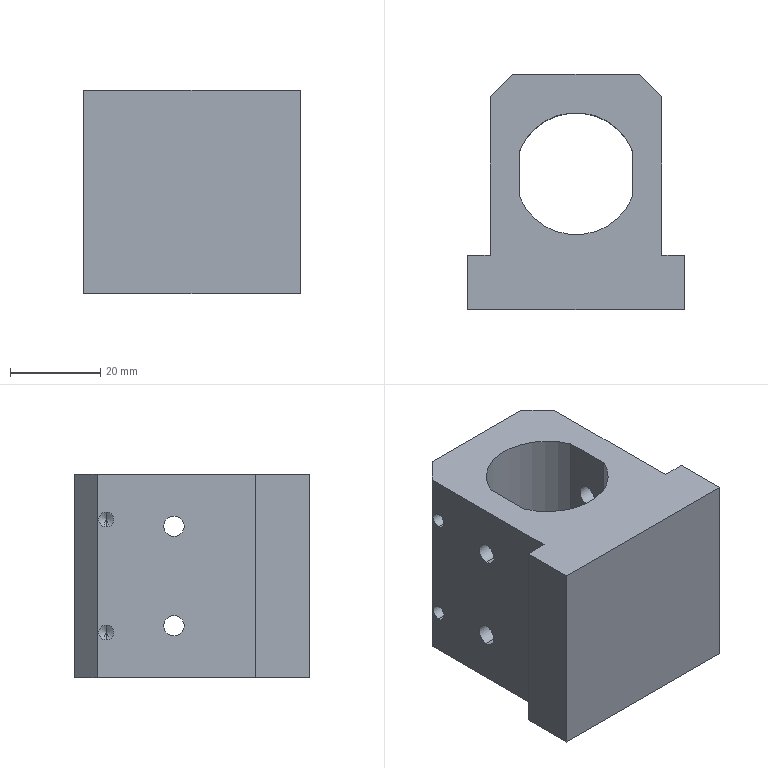Part | STEP file | detection slider--1 | 1 solid | 56 faces | box 48 x 52 x 45 mm | volume 66698 mm3 | cylinder 26 | cone 16 | plane 14 | commonest cylinder face diameters 3.3 x12 4.5 x8 4.2 x4 27 x2